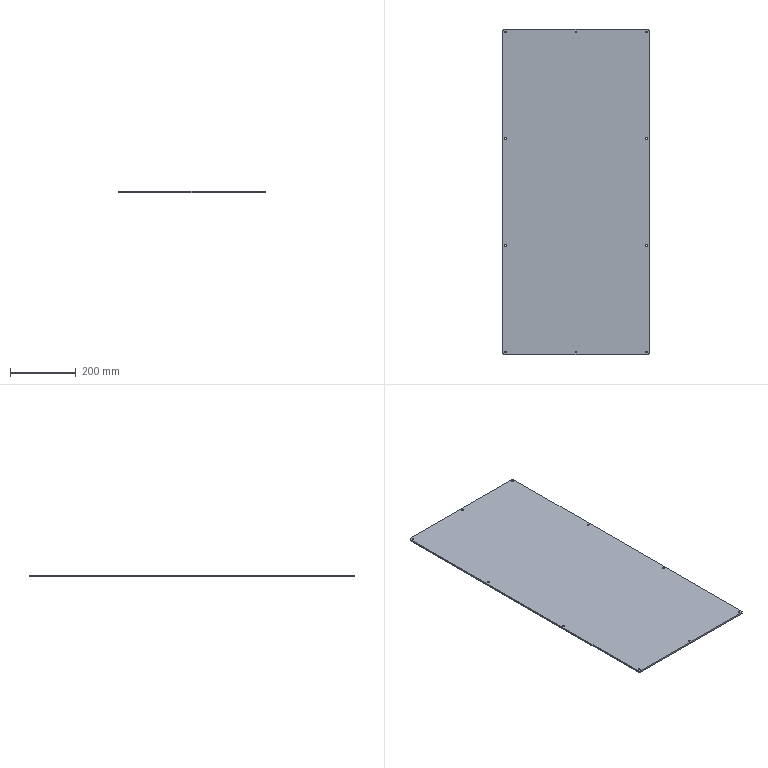Part | NX | features BREP 1 | 1 solid | 30 faces | box 446 x 992 x 5 mm | volume 2210732 mm3 | cylinder 24 | plane 6 | commonest cylinder face diameters 5.8 x20 10 x4
STEP:
#1=CARTESIAN_POINT('',(-218.,496.,5.));
#2=VERTEX_POINT('',#1);
#3=CARTESIAN_POINT('',(-223.,491.,5.));
#4=VERTEX_POINT('',#3);
#5=CARTESIAN_POINT('',(-218.,491.,5.));
#6=DIRECTION('',(0.,0.,1.));
#7=DIRECTION('',(1.,0.,0.));
#8=AXIS2_PLACEMENT_3D('',#5,#6,#7);
#9=CIRCLE('',#8,5.);
#10=EDGE_CURVE('',#2,#4,#9,.T.);
#11=ORIENTED_EDGE('',*,*,#10,.F.);
#12=CARTESIAN_POINT('',(-218.,496.,0.));
#13=VERTEX_POINT('',#12);
#14=CARTESIAN_POINT('',(-218.,496.,5.));
#15=DIRECTION('',(0.,0.,1.));
#16=VECTOR('',#15,1000.);
#17=LINE('',#14,#16);
#18=EDGE_CURVE('',#13,#2,#17,.T.);
#19=ORIENTED_EDGE('',*,*,#18,.F.);
#20=CARTESIAN_POINT('',(-223.,491.,0.));
#21=VERTEX_POINT('',#20);
#22=CARTESIAN_POINT('',(-218.,491.,0.));
#23=DIRECTION('',(0.,0.,-1.));
#24=DIRECTION('',(1.,0.,0.));
#25=AXIS2_PLACEMENT_3D('',#22,#23,#24);
#26=CIRCLE('',#25,5.);
#27=EDGE_CURVE('',#21,#13,#26,.T.);
#28=ORIENTED_EDGE('',*,*,#27,.F.);
#29=CARTESIAN_POINT('',(-223.,491.,5.));
#30=DIRECTION('',(0.,0.,-1.));
#31=VECTOR('',#30,1000.);
#32=LINE('',#29,#31);
#33=EDGE_CURVE('',#4,#21,#32,.T.);
#34=ORIENTED_EDGE('',*,*,#33,.F.);
#35=EDGE_LOOP('',(#11,#19,#28,#34));
#36=FACE_BOUND('',#35,.T.);
#37=CARTESIAN_POINT('',(-218.,491.,5.));
#38=DIRECTION('',(0.,0.,-1.));
#39=DIRECTION('',(-1.,0.,0.));
#40=AXIS2_PLACEMENT_3D('',#37,#38,#39);
#41=CYLINDRICAL_SURFACE('',#40,5.);
#42=ADVANCED_FACE('',(#36),#41,.T.);
#43=CARTESIAN_POINT('',(223.,491.,5.));
#44=VERTEX_POINT('',#43);
#45=CARTESIAN_POINT('',(218.,496.,5.));
#46=VERTEX_POINT('',#45);
#47=CARTESIAN_POINT('',(218.,491.,5.));
#48=DIRECTION('',(0.,0.,1.));
#49=DIRECTION('',(1.,0.,0.));
#50=AXIS2_PLACEMENT_3D('',#47,#48,#49);
#51=CIRCLE('',#50,5.);
#52=EDGE_CURVE('',#44,#46,#51,.T.);
#53=ORIENTED_EDGE('',*,*,#52,.F.);
#54=CARTESIAN_POINT('',(223.,491.,0.));
#55=VERTEX_POINT('',#54);
#56=CARTESIAN_POINT('',(223.,491.,5.));
#57=DIRECTION('',(0.,0.,1.));
#58=VECTOR('',#57,1000.);
#59=LINE('',#56,#58);
#60=EDGE_CURVE('',#55,#44,#59,.T.);
#61=ORIENTED_EDGE('',*,*,#60,.F.);
#62=CARTESIAN_POINT('',(218.,496.,0.));
#63=VERTEX_POINT('',#62);
#64=CARTESIAN_POINT('',(218.,491.,0.));
#65=DIRECTION('',(0.,0.,-1.));
#66=DIRECTION('',(1.,0.,0.));
#67=AXIS2_PLACEMENT_3D('',#64,#65,#66);
#68=CIRCLE('',#67,5.);
#69=EDGE_CURVE('',#63,#55,#68,.T.);
#70=ORIENTED_EDGE('',*,*,#69,.F.);
#71=CARTESIAN_POINT('',(218.,496.,5.));
#72=DIRECTION('',(0.,0.,-1.));
#73=VECTOR('',#72,1000.);
#74=LINE('',#71,#73);
#75=EDGE_CURVE('',#46,#63,#74,.T.);
#76=ORIENTED_EDGE('',*,*,#75,.F.);
#77=EDGE_LOOP('',(#53,#61,#70,#76));
#78=FACE_BOUND('',#77,.T.);
#79=CARTESIAN_POINT('',(218.,491.,5.));
#80=DIRECTION('',(0.,0.,-1.));
#81=DIRECTION('',(-1.,0.,0.));
#82=AXIS2_PLACEMENT_3D('',#79,#80,#81);
#83=CYLINDRICAL_SURFACE('',#82,5.);
#84=ADVANCED_FACE('',(#78),#83,.T.);
#85=CARTESIAN_POINT('',(218.,-496.,5.));
#86=VERTEX_POINT('',#85);
#87=CARTESIAN_POINT('',(223.,-491.,5.));
#88=VERTEX_POINT('',#87);
#89=CARTESIAN_POINT('',(218.,-491.,5.));
#90=DIRECTION('',(0.,0.,1.));
#91=DIRECTION('',(1.,0.,0.));
#92=AXIS2_PLACEMENT_3D('',#89,#90,#91);
#93=CIRCLE('',#92,5.);
#94=EDGE_CURVE('',#86,#88,#93,.T.);
#95=ORIENTED_EDGE('',*,*,#94,.F.);
#96=CARTESIAN_POINT('',(218.,-496.,0.));
#97=VERTEX_POINT('',#96);
#98=CARTESIAN_POINT('',(218.,-496.,5.));
#99=DIRECTION('',(0.,0.,1.));
#100=VECTOR('',#99,1000.);
#101=LINE('',#98,#100);
#102=EDGE_CURVE('',#97,#86,#101,.T.);
#103=ORIENTED_EDGE('',*,*,#102,.F.);
#104=CARTESIAN_POINT('',(223.,-491.,0.));
#105=VERTEX_POINT('',#104);
#106=CARTESIAN_POINT('',(218.,-491.,0.));
#107=DIRECTION('',(0.,0.,-1.));
#108=DIRECTION('',(1.,0.,0.));
#109=AXIS2_PLACEMENT_3D('',#106,#107,#108);
#110=CIRCLE('',#109,5.);
#111=EDGE_CURVE('',#105,#97,#110,.T.);
#112=ORIENTED_EDGE('',*,*,#111,.F.);
#113=CARTESIAN_POINT('',(223.,-491.,5.));
#114=DIRECTION('',(0.,0.,-1.));
#115=VECTOR('',#114,1000.);
#116=LINE('',#113,#115);
#117=EDGE_CURVE('',#88,#105,#116,.T.);
#118=ORIENTED_EDGE('',*,*,#117,.F.);
#119=EDGE_LOOP('',(#95,#103,#112,#118));
#120=FACE_BOUND('',#119,.T.);
#121=CARTESIAN_POINT('',(218.,-491.,5.));
#122=DIRECTION('',(0.,0.,-1.));
#123=DIRECTION('',(-1.,0.,0.));
#124=AXIS2_PLACEMENT_3D('',#121,#122,#123);
#125=CYLINDRICAL_SURFACE('',#124,5.);
#126=ADVANCED_FACE('',(#120),#125,.T.);
#127=CARTESIAN_POINT('',(-223.,-491.,5.));
#128=VERTEX_POINT('',#127);
#129=CARTESIAN_POINT('',(-218.,-496.,5.));
#130=VERTEX_POINT('',#129);
#131=CARTESIAN_POINT('',(-218.,-491.,5.));
#132=DIRECTION('',(0.,0.,1.));
#133=DIRECTION('',(1.,0.,0.));
#134=AXIS2_PLACEMENT_3D('',#131,#132,#133);
#135=CIRCLE('',#134,5.);
#136=EDGE_CURVE('',#128,#130,#135,.T.);
#137=ORIENTED_EDGE('',*,*,#136,.F.);
#138=CARTESIAN_POINT('',(-223.,-491.,0.));
#139=VERTEX_POINT('',#138);
#140=CARTESIAN_POINT('',(-223.,-491.,5.));
#141=DIRECTION('',(0.,0.,1.));
#142=VECTOR('',#141,1000.);
#143=LINE('',#140,#142);
#144=EDGE_CURVE('',#139,#128,#143,.T.);
#145=ORIENTED_EDGE('',*,*,#144,.F.);
#146=CARTESIAN_POINT('',(-218.,-496.,0.));
#147=VERTEX_POINT('',#146);
#148=CARTESIAN_POINT('',(-218.,-491.,0.));
#149=DIRECTION('',(0.,0.,-1.));
#150=DIRECTION('',(1.,0.,0.));
#151=AXIS2_PLACEMENT_3D('',#148,#149,#150);
#152=CIRCLE('',#151,5.);
#153=EDGE_CURVE('',#147,#139,#152,.T.);
#154=ORIENTED_EDGE('',*,*,#153,.F.);
#155=CARTESIAN_POINT('',(-218.,-496.,5.));
#156=DIRECTION('',(0.,0.,-1.));
#157=VECTOR('',#156,1000.);
#158=LINE('',#155,#157);
#159=EDGE_CURVE('',#130,#147,#158,.T.);
#160=ORIENTED_EDGE('',*,*,#159,.F.);
#161=EDGE_LOOP('',(#137,#145,#154,#160));
#162=FACE_BOUND('',#161,.T.);
#163=CARTESIAN_POINT('',(-218.,-491.,5.));
#164=DIRECTION('',(0.,0.,-1.));
#165=DIRECTION('',(-1.,0.,0.));
#166=AXIS2_PLACEMENT_3D('',#163,#164,#165);
#167=CYLINDRICAL_SURFACE('',#166,5.);
#168=ADVANCED_FACE('',(#162),#167,.T.);
#169=CARTESIAN_POINT('',(212.1,-488.,5.));
#170=VERTEX_POINT('',#169);
#171=CARTESIAN_POINT('',(212.1,-488.,0.));
#172=VERTEX_POINT('',#171);
#173=CARTESIAN_POINT('',(212.1,-488.,0.));
#174=DIRECTION('',(0.,0.,1.));
#175=VECTOR('',#174,1000.);
#176=LINE('',#173,#175);
#177=EDGE_CURVE('',#170,#172,#176,.F.);
#178=ORIENTED_EDGE('',*,*,#177,.T.);
#179=CARTESIAN_POINT('',(217.9,-488.,0.));
#180=VERTEX_POINT('',#179);
#181=CARTESIAN_POINT('',(215.,-488.,0.));
#182=DIRECTION('',(0.,0.,1.));
#183=DIRECTION('',(1.,0.,0.));
#184=AXIS2_PLACEMENT_3D('',#181,#182,#183);
#185=CIRCLE('',#184,2.9);
#186=EDGE_CURVE('',#180,#172,#185,.T.);
#187=ORIENTED_EDGE('',*,*,#186,.F.);
#188=CARTESIAN_POINT('',(217.9,-488.,5.));
#189=VERTEX_POINT('',#188);
#190=CARTESIAN_POINT('',(217.9,-488.,0.));
#191=DIRECTION('',(0.,0.,1.));
#192=VECTOR('',#191,1000.);
#193=LINE('',#190,#192);
#194=EDGE_CURVE('',#189,#180,#193,.F.);
#195=ORIENTED_EDGE('',*,*,#194,.F.);
#196=CARTESIAN_POINT('',(215.,-488.,5.));
#197=DIRECTION('',(0.,0.,1.));
#198=DIRECTION('',(1.,0.,0.));
#199=AXIS2_PLACEMENT_3D('',#196,#197,#198);
#200=CIRCLE('',#199,2.9);
#201=EDGE_CURVE('',#189,#170,#200,.T.);
#202=ORIENTED_EDGE('',*,*,#201,.T.);
#203=EDGE_LOOP('',(#178,#187,#195,#202));
#204=FACE_BOUND('',#203,.T.);
#205=CARTESIAN_POINT('',(215.,-488.,0.));
#206=DIRECTION('',(0.,0.,1.));
#207=DIRECTION('',(1.,0.,0.));
#208=AXIS2_PLACEMENT_3D('',#205,#206,#207);
#209=CYLINDRICAL_SURFACE('',#208,2.9);
#210=ADVANCED_FACE('',(#204),#209,.F.);
#211=CARTESIAN_POINT('',(212.1,162.667,5.));
#212=VERTEX_POINT('',#211);
#213=CARTESIAN_POINT('',(212.1,162.667,0.));
#214=VERTEX_POINT('',#213);
#215=CARTESIAN_POINT('',(212.1,162.667,0.));
#216=DIRECTION('',(0.,0.,1.));
#217=VECTOR('',#216,1000.);
#218=LINE('',#215,#217);
#219=EDGE_CURVE('',#212,#214,#218,.F.);
#220=ORIENTED_EDGE('',*,*,#219,.T.);
#221=CARTESIAN_POINT('',(217.9,162.667,0.));
#222=VERTEX_POINT('',#221);
#223=CARTESIAN_POINT('',(215.,162.667,0.));
#224=DIRECTION('',(0.,0.,1.));
#225=DIRECTION('',(1.,0.,0.));
#226=AXIS2_PLACEMENT_3D('',#223,#224,#225);
#227=CIRCLE('',#226,2.9);
#228=EDGE_CURVE('',#222,#214,#227,.T.);
#229=ORIENTED_EDGE('',*,*,#228,.F.);
#230=CARTESIAN_POINT('',(217.9,162.667,5.));
#231=VERTEX_POINT('',#230);
#232=CARTESIAN_POINT('',(217.9,162.667,0.));
#233=DIRECTION('',(0.,0.,1.));
#234=VECTOR('',#233,1000.);
#235=LINE('',#232,#234);
#236=EDGE_CURVE('',#231,#222,#235,.F.);
#237=ORIENTED_EDGE('',*,*,#236,.F.);
#238=CARTESIAN_POINT('',(215.,162.667,5.));
#239=DIRECTION('',(0.,0.,1.));
#240=DIRECTION('',(1.,0.,0.));
#241=AXIS2_PLACEMENT_3D('',#238,#239,#240);
#242=CIRCLE('',#241,2.9);
#243=EDGE_CURVE('',#231,#212,#242,.T.);
#244=ORIENTED_EDGE('',*,*,#243,.T.);
#245=EDGE_LOOP('',(#220,#229,#237,#244));
#246=FACE_BOUND('',#245,.T.);
#247=CARTESIAN_POINT('',(215.,162.667,0.));
#248=DIRECTION('',(0.,0.,1.));
#249=DIRECTION('',(1.,0.,0.));
#250=AXIS2_PLACEMENT_3D('',#247,#248,#249);
#251=CYLINDRICAL_SURFACE('',#250,2.9);
#252=ADVANCED_FACE('',(#246),#251,.F.);
#253=CARTESIAN_POINT('',(212.1,-162.667,5.));
#254=VERTEX_POINT('',#253);
#255=CARTESIAN_POINT('',(212.1,-162.667,0.));
#256=VERTEX_POINT('',#255);
#257=CARTESIAN_POINT('',(212.1,-162.667,0.));
#258=DIRECTION('',(0.,0.,1.));
#259=VECTOR('',#258,1000.);
#260=LINE('',#257,#259);
#261=EDGE_CURVE('',#254,#256,#260,.F.);
#262=ORIENTED_EDGE('',*,*,#261,.T.);
#263=CARTESIAN_POINT('',(217.9,-162.667,0.));
#264=VERTEX_POINT('',#263);
#265=CARTESIAN_POINT('',(215.,-162.667,0.));
#266=DIRECTION('',(0.,0.,1.));
#267=DIRECTION('',(1.,0.,0.));
#268=AXIS2_PLACEMENT_3D('',#265,#266,#267);
#269=CIRCLE('',#268,2.9);
#270=EDGE_CURVE('',#264,#256,#269,.T.);
#271=ORIENTED_EDGE('',*,*,#270,.F.);
#272=CARTESIAN_POINT('',(217.9,-162.667,5.));
#273=VERTEX_POINT('',#272);
#274=CARTESIAN_POINT('',(217.9,-162.667,0.));
#275=DIRECTION('',(0.,0.,1.));
#276=VECTOR('',#275,1000.);
#277=LINE('',#274,#276);
#278=EDGE_CURVE('',#273,#264,#277,.F.);
#279=ORIENTED_EDGE('',*,*,#278,.F.);
#280=CARTESIAN_POINT('',(215.,-162.667,5.));
#281=DIRECTION('',(0.,0.,1.));
#282=DIRECTION('',(1.,0.,0.));
#283=AXIS2_PLACEMENT_3D('',#280,#281,#282);
#284=CIRCLE('',#283,2.9);
#285=EDGE_CURVE('',#273,#254,#284,.T.);
#286=ORIENTED_EDGE('',*,*,#285,.T.);
#287=EDGE_LOOP('',(#262,#271,#279,#286));
#288=FACE_BOUND('',#287,.T.);
#289=CARTESIAN_POINT('',(215.,-162.667,0.));
#290=DIRECTION('',(0.,0.,1.));
#291=DIRECTION('',(1.,0.,0.));
#292=AXIS2_PLACEMENT_3D('',#289,#290,#291);
#293=CYLINDRICAL_SURFACE('',#292,2.9);
#294=ADVANCED_FACE('',(#288),#293,.F.);
#295=CARTESIAN_POINT('',(-217.9,162.667,5.));
#296=VERTEX_POINT('',#295);
#297=CARTESIAN_POINT('',(-217.9,162.667,0.));
#298=VERTEX_POINT('',#297);
#299=CARTESIAN_POINT('',(-217.9,162.667,0.));
#300=DIRECTION('',(0.,0.,1.));
#301=VECTOR('',#300,1000.);
#302=LINE('',#299,#301);
#303=EDGE_CURVE('',#296,#298,#302,.F.);
#304=ORIENTED_EDGE('',*,*,#303,.T.);
#305=CARTESIAN_POINT('',(-212.1,162.667,0.));
#306=VERTEX_POINT('',#305);
#307=CARTESIAN_POINT('',(-215.,162.667,0.));
#308=DIRECTION('',(0.,0.,1.));
#309=DIRECTION('',(1.,0.,0.));
#310=AXIS2_PLACEMENT_3D('',#307,#308,#309);
#311=CIRCLE('',#310,2.9);
#312=EDGE_CURVE('',#306,#298,#311,.T.);
#313=ORIENTED_EDGE('',*,*,#312,.F.);
#314=CARTESIAN_POINT('',(-212.1,162.667,5.));
#315=VERTEX_POINT('',#314);
#316=CARTESIAN_POINT('',(-212.1,162.667,0.));
#317=DIRECTION('',(0.,0.,1.));
#318=VECTOR('',#317,1000.);
#319=LINE('',#316,#318);
#320=EDGE_CURVE('',#315,#306,#319,.F.);
#321=ORIENTED_EDGE('',*,*,#320,.F.);
#322=CARTESIAN_POINT('',(-215.,162.667,5.));
#323=DIRECTION('',(0.,0.,1.));
#324=DIRECTION('',(1.,0.,0.));
#325=AXIS2_PLACEMENT_3D('',#322,#323,#324);
#326=CIRCLE('',#325,2.9);
#327=EDGE_CURVE('',#315,#296,#326,.T.);
#328=ORIENTED_EDGE('',*,*,#327,.T.);
#329=EDGE_LOOP('',(#304,#313,#321,#328));
#330=FACE_BOUND('',#329,.T.);
#331=CARTESIAN_POINT('',(-215.,162.667,0.));
#332=DIRECTION('',(0.,0.,1.));
#333=DIRECTION('',(1.,0.,0.));
#334=AXIS2_PLACEMENT_3D('',#331,#332,#333);
#335=CYLINDRICAL_SURFACE('',#334,2.9);
#336=ADVANCED_FACE('',(#330),#335,.F.);
#337=CARTESIAN_POINT('',(-2.9,-488.,5.));
#338=VERTEX_POINT('',#337);
#339=CARTESIAN_POINT('',(-2.9,-488.,0.));
#340=VERTEX_POINT('',#339);
#341=CARTESIAN_POINT('',(-2.9,-488.,0.));
#342=DIRECTION('',(0.,0.,1.));
#343=VECTOR('',#342,1000.);
#344=LINE('',#341,#343);
#345=EDGE_CURVE('',#338,#340,#344,.F.);
#346=ORIENTED_EDGE('',*,*,#345,.T.);
#347=CARTESIAN_POINT('',(2.9,-488.,0.));
#348=VERTEX_POINT('',#347);
#349=CARTESIAN_POINT('',(0.,-488.,0.));
#350=DIRECTION('',(0.,0.,1.));
#351=DIRECTION('',(1.,0.,0.));
#352=AXIS2_PLACEMENT_3D('',#349,#350,#351);
#353=CIRCLE('',#352,2.9);
#354=EDGE_CURVE('',#348,#340,#353,.T.);
#355=ORIENTED_EDGE('',*,*,#354,.F.);
#356=CARTESIAN_POINT('',(2.9,-488.,5.));
#357=VERTEX_POINT('',#356);
#358=CARTESIAN_POINT('',(2.9,-488.,0.));
#359=DIRECTION('',(0.,0.,1.));
#360=VECTOR('',#359,1000.);
#361=LINE('',#358,#360);
#362=EDGE_CURVE('',#357,#348,#361,.F.);
#363=ORIENTED_EDGE('',*,*,#362,.F.);
#364=CARTESIAN_POINT('',(0.,-488.,5.));
#365=DIRECTION('',(0.,0.,1.));
#366=DIRECTION('',(1.,0.,0.));
#367=AXIS2_PLACEMENT_3D('',#364,#365,#366);
#368=CIRCLE('',#367,2.9);
#369=EDGE_CURVE('',#357,#338,#368,.T.);
#370=ORIENTED_EDGE('',*,*,#369,.T.);
#371=EDGE_LOOP('',(#346,#355,#363,#370));
#372=FACE_BOUND('',#371,.T.);
#373=CARTESIAN_POINT('',(0.,-488.,0.));
#374=DIRECTION('',(0.,0.,1.));
#375=DIRECTION('',(1.,0.,0.));
#376=AXIS2_PLACEMENT_3D('',#373,#374,#375);
#377=CYLINDRICAL_SURFACE('',#376,2.9);
#378=ADVANCED_FACE('',(#372),#377,.F.);
#379=CARTESIAN_POINT('',(-217.9,-488.,5.));
#380=VERTEX_POINT('',#379);
#381=CARTESIAN_POINT('',(-217.9,-488.,0.));
#382=VERTEX_POINT('',#381);
#383=CARTESIAN_POINT('',(-217.9,-488.,0.));
#384=DIRECTION('',(0.,0.,1.));
#385=VECTOR('',#384,1000.);
#386=LINE('',#383,#385);
#387=EDGE_CURVE('',#380,#382,#386,.F.);
#388=ORIENTED_EDGE('',*,*,#387,.T.);
#389=CARTESIAN_POINT('',(-212.1,-488.,0.));
#390=VERTEX_POINT('',#389);
#391=CARTESIAN_POINT('',(-215.,-488.,0.));
#392=DIRECTION('',(0.,0.,1.));
#393=DIRECTION('',(1.,0.,0.));
#394=AXIS2_PLACEMENT_3D('',#391,#392,#393);
#395=CIRCLE('',#394,2.9);
#396=EDGE_CURVE('',#390,#382,#395,.T.);
#397=ORIENTED_EDGE('',*,*,#396,.F.);
#398=CARTESIAN_POINT('',(-212.1,-488.,5.));
#399=VERTEX_POINT('',#398);
#400=CARTESIAN_POINT('',(-212.1,-488.,0.));
#401=DIRECTION('',(0.,0.,1.));
#402=VECTOR('',#401,1000.);
#403=LINE('',#400,#402);
#404=EDGE_CURVE('',#399,#390,#403,.F.);
#405=ORIENTED_EDGE('',*,*,#404,.F.);
#406=CARTESIAN_POINT('',(-215.,-488.,5.));
#407=DIRECTION('',(0.,0.,1.));
#408=DIRECTION('',(1.,0.,0.));
#409=AXIS2_PLACEMENT_3D('',#406,#407,#408);
#410=CIRCLE('',#409,2.9);
#411=EDGE_CURVE('',#399,#380,#410,.T.);
#412=ORIENTED_EDGE('',*,*,#411,.T.);
#413=EDGE_LOOP('',(#388,#397,#405,#412));
#414=FACE_BOUND('',#413,.T.);
#415=CARTESIAN_POINT('',(-215.,-488.,0.));
#416=DIRECTION('',(0.,0.,1.));
#417=DIRECTION('',(1.,0.,0.));
#418=AXIS2_PLACEMENT_3D('',#415,#416,#417);
#419=CYLINDRICAL_SURFACE('',#418,2.9);
#420=ADVANCED_FACE('',(#414),#419,.F.);
#421=CARTESIAN_POINT('',(212.1,488.,5.));
#422=VERTEX_POINT('',#421);
#423=CARTESIAN_POINT('',(212.1,488.,0.));
#424=VERTEX_POINT('',#423);
#425=CARTESIAN_POINT('',(212.1,488.,0.));
#426=DIRECTION('',(0.,0.,1.));
#427=VECTOR('',#426,1000.);
#428=LINE('',#425,#427);
#429=EDGE_CURVE('',#422,#424,#428,.F.);
#430=ORIENTED_EDGE('',*,*,#429,.T.);
#431=CARTESIAN_POINT('',(217.9,488.,0.));
#432=VERTEX_POINT('',#431);
#433=CARTESIAN_POINT('',(215.,488.,0.));
#434=DIRECTION('',(0.,0.,1.));
#435=DIRECTION('',(1.,0.,0.));
#436=AXIS2_PLACEMENT_3D('',#433,#434,#435);
#437=CIRCLE('',#436,2.9);
#438=EDGE_CURVE('',#432,#424,#437,.T.);
#439=ORIENTED_EDGE('',*,*,#438,.F.);
#440=CARTESIAN_POINT('',(217.9,488.,5.));
#441=VERTEX_POINT('',#440);
#442=CARTESIAN_POINT('',(217.9,488.,0.));
#443=DIRECTION('',(0.,0.,1.));
#444=VECTOR('',#443,1000.);
#445=LINE('',#442,#444);
#446=EDGE_CURVE('',#441,#432,#445,.F.);
#447=ORIENTED_EDGE('',*,*,#446,.F.);
#448=CARTESIAN_POINT('',(215.,488.,5.));
#449=DIRECTION('',(0.,0.,1.));
#450=DIRECTION('',(1.,0.,0.));
#451=AXIS2_PLACEMENT_3D('',#448,#449,#450);
#452=CIRCLE('',#451,2.9);
#453=EDGE_CURVE('',#441,#422,#452,.T.);
#454=ORIENTED_EDGE('',*,*,#453,.T.);
#455=EDGE_LOOP('',(#430,#439,#447,#454));
#456=FACE_BOUND('',#455,.T.);
#457=CARTESIAN_POINT('',(215.,488.,0.));
#458=DIRECTION('',(0.,0.,1.));
#459=DIRECTION('',(1.,0.,0.));
#460=AXIS2_PLACEMENT_3D('',#457,#458,#459);
#461=CYLINDRICAL_SURFACE('',#460,2.9);
#462=ADVANCED_FACE('',(#456),#461,.F.);
#463=CARTESIAN_POINT('',(-2.9,488.,5.));
#464=VERTEX_POINT('',#463);
#465=CARTESIAN_POINT('',(-2.9,488.,0.));
#466=VERTEX_POINT('',#465);
#467=CARTESIAN_POINT('',(-2.9,488.,0.));
#468=DIRECTION('',(0.,0.,1.));
#469=VECTOR('',#468,1000.);
#470=LINE('',#467,#469);
#471=EDGE_CURVE('',#464,#466,#470,.F.);
#472=ORIENTED_EDGE('',*,*,#471,.T.);
#473=CARTESIAN_POINT('',(2.9,488.,0.));
#474=VERTEX_POINT('',#473);
#475=CARTESIAN_POINT('',(0.,488.,0.));
#476=DIRECTION('',(0.,0.,1.));
#477=DIRECTION('',(1.,0.,0.));
#478=AXIS2_PLACEMENT_3D('',#475,#476,#477);
#479=CIRCLE('',#478,2.9);
#480=EDGE_CURVE('',#474,#466,#479,.T.);
#481=ORIENTED_EDGE('',*,*,#480,.F.);
#482=CARTESIAN_POINT('',(2.9,488.,5.));
#483=VERTEX_POINT('',#482);
#484=CARTESIAN_POINT('',(2.9,488.,0.));
#485=DIRECTION('',(0.,0.,1.));
#486=VECTOR('',#485,1000.);
#487=LINE('',#484,#486);
#488=EDGE_CURVE('',#483,#474,#487,.F.);
#489=ORIENTED_EDGE('',*,*,#488,.F.);
#490=CARTESIAN_POINT('',(0.,488.,5.));
#491=DIRECTION('',(0.,0.,1.));
#492=DIRECTION('',(1.,0.,0.));
#493=AXIS2_PLACEMENT_3D('',#490,#491,#492);
#494=CIRCLE('',#493,2.9);
#495=EDGE_CURVE('',#483,#464,#494,.T.);
#496=ORIENTED_EDGE('',*,*,#495,.T.);
#497=EDGE_LOOP('',(#472,#481,#489,#496));
#498=FACE_BOUND('',#497,.T.);
#499=CARTESIAN_POINT('',(0.,488.,0.));
#500=DIRECTION('',(0.,0.,1.));
#501=DIRECTION('',(1.,0.,0.));
#502=AXIS2_PLACEMENT_3D('',#499,#500,#501);
#503=CYLINDRICAL_SURFACE('',#502,2.9);
#504=ADVANCED_FACE('',(#498),#503,.F.);
#505=CARTESIAN_POINT('',(-217.9,-162.667,5.));
#506=VERTEX_POINT('',#505);
#507=CARTESIAN_POINT('',(-217.9,-162.667,0.));
#508=VERTEX_POINT('',#507);
#509=CARTESIAN_POINT('',(-217.9,-162.667,0.));
#510=DIRECTION('',(0.,0.,1.));
#511=VECTOR('',#510,1000.);
#512=LINE('',#509,#511);
#513=EDGE_CURVE('',#506,#508,#512,.F.);
#514=ORIENTED_EDGE('',*,*,#513,.T.);
#515=CARTESIAN_POINT('',(-212.1,-162.667,0.));
#516=VERTEX_POINT('',#515);
#517=CARTESIAN_POINT('',(-215.,-162.667,0.));
#518=DIRECTION('',(0.,0.,1.));
#519=DIRECTION('',(1.,0.,0.));
#520=AXIS2_PLACEMENT_3D('',#517,#518,#519);
#521=CIRCLE('',#520,2.9);
#522=EDGE_CURVE('',#516,#508,#521,.T.);
#523=ORIENTED_EDGE('',*,*,#522,.F.);
#524=CARTESIAN_POINT('',(-212.1,-162.667,5.));
#525=VERTEX_POINT('',#524);
#526=CARTESIAN_POINT('',(-212.1,-162.667,0.));
#527=DIRECTION('',(0.,0.,1.));
#528=VECTOR('',#527,1000.);
#529=LINE('',#526,#528);
#530=EDGE_CURVE('',#525,#516,#529,.F.);
#531=ORIENTED_EDGE('',*,*,#530,.F.);
#532=CARTESIAN_POINT('',(-215.,-162.667,5.));
#533=DIRECTION('',(0.,0.,1.));
#534=DIRECTION('',(1.,0.,0.));
#535=AXIS2_PLACEMENT_3D('',#532,#533,#534);
#536=CIRCLE('',#535,2.9);
#537=EDGE_CURVE('',#525,#506,#536,.T.);
#538=ORIENTED_EDGE('',*,*,#537,.T.);
#539=EDGE_LOOP('',(#514,#523,#531,#538));
#540=FACE_BOUND('',#539,.T.);
#541=CARTESIAN_POINT('',(-215.,-162.667,0.));
#542=DIRECTION('',(0.,0.,1.));
#543=DIRECTION('',(1.,0.,0.));
#544=AXIS2_PLACEMENT_3D('',#541,#542,#543);
#545=CYLINDRICAL_SURFACE('',#544,2.9);
#546=ADVANCED_FACE('',(#540),#545,.F.);
#547=CARTESIAN_POINT('',(-217.9,488.,5.));
#548=VERTEX_POINT('',#547);
#549=CARTESIAN_POINT('',(-217.9,488.,0.));
#550=VERTEX_POINT('',#549);
#551=CARTESIAN_POINT('',(-217.9,488.,0.));
#552=DIRECTION('',(0.,0.,1.));
#553=VECTOR('',#552,1000.);
#554=LINE('',#551,#553);
#555=EDGE_CURVE('',#548,#550,#554,.F.);
#556=ORIENTED_EDGE('',*,*,#555,.T.);
#557=CARTESIAN_POINT('',(-212.1,488.,0.));
#558=VERTEX_POINT('',#557);
#559=CARTESIAN_POINT('',(-215.,488.,0.));
#560=DIRECTION('',(0.,0.,1.));
#561=DIRECTION('',(1.,0.,0.));
#562=AXIS2_PLACEMENT_3D('',#559,#560,#561);
#563=CIRCLE('',#562,2.9);
#564=EDGE_CURVE('',#558,#550,#563,.T.);
#565=ORIENTED_EDGE('',*,*,#564,.F.);
#566=CARTESIAN_POINT('',(-212.1,488.,5.));
#567=VERTEX_POINT('',#566);
#568=CARTESIAN_POINT('',(-212.1,488.,0.));
#569=DIRECTION('',(0.,0.,1.));
#570=VECTOR('',#569,1000.);
#571=LINE('',#568,#570);
#572=EDGE_CURVE('',#567,#558,#571,.F.);
#573=ORIENTED_EDGE('',*,*,#572,.F.);
#574=CARTESIAN_POINT('',(-215.,488.,5.));
#575=DIRECTION('',(0.,0.,1.));
#576=DIRECTION('',(1.,0.,0.));
#577=AXIS2_PLACEMENT_3D('',#574,#575,#576);
#578=CIRCLE('',#577,2.9);
#579=EDGE_CURVE('',#567,#548,#578,.T.);
#580=ORIENTED_EDGE('',*,*,#579,.T.);
#581=EDGE_LOOP('',(#556,#565,#573,#580));
#582=FACE_BOUND('',#581,.T.);
#583=CARTESIAN_POINT('',(-215.,488.,0.));
#584=DIRECTION('',(0.,0.,1.));
#585=DIRECTION('',(1.,0.,0.));
#586=AXIS2_PLACEMENT_3D('',#583,#584,#585);
#587=CYLINDRICAL_SURFACE('',#586,2.9);
#588=ADVANCED_FACE('',(#582),#587,.F.);
#589=CARTESIAN_POINT('',(223.,-496.,0.));
#590=DIRECTION('',(1.,0.,0.));
#591=VECTOR('',#590,1000.);
#592=LINE('',#589,#591);
#593=EDGE_CURVE('',#147,#97,#592,.T.);
#594=ORIENTED_EDGE('',*,*,#593,.F.);
#595=ORIENTED_EDGE('',*,*,#153,.T.);
#596=CARTESIAN_POINT('',(-223.,-496.,0.));
#597=DIRECTION('',(0.,-1.,0.));
#598=VECTOR('',#597,1000.);
#599=LINE('',#596,#598);
#600=EDGE_CURVE('',#21,#139,#599,.T.);
#601=ORIENTED_EDGE('',*,*,#600,.F.);
#602=ORIENTED_EDGE('',*,*,#27,.T.);
#603=CARTESIAN_POINT('',(223.,496.,0.));
#604=DIRECTION('',(-1.,0.,0.));
#605=VECTOR('',#604,1000.);
#606=LINE('',#603,#605);
#607=EDGE_CURVE('',#63,#13,#606,.T.);
#608=ORIENTED_EDGE('',*,*,#607,.F.);
#609=ORIENTED_EDGE('',*,*,#69,.T.);
#610=CARTESIAN_POINT('',(223.,-496.,0.));
#611=DIRECTION('',(0.,1.,0.));
#612=VECTOR('',#611,1000.);
#613=LINE('',#610,#612);
#614=EDGE_CURVE('',#105,#55,#613,.T.);
#615=ORIENTED_EDGE('',*,*,#614,.F.);
#616=ORIENTED_EDGE('',*,*,#111,.T.);
#617=EDGE_LOOP('',(#594,#595,#601,#602,#608,#609,#615,#616));
#618=FACE_BOUND('',#617,.T.);
#619=ORIENTED_EDGE('',*,*,#564,.T.);
#620=CARTESIAN_POINT('',(-215.,488.,0.));
#621=DIRECTION('',(0.,0.,1.));
#622=DIRECTION('',(1.,0.,0.));
#623=AXIS2_PLACEMENT_3D('',#620,#621,#622);
#624=CIRCLE('',#623,2.9);
#625=EDGE_CURVE('',#550,#558,#624,.T.);
#626=ORIENTED_EDGE('',*,*,#625,.T.);
#627=EDGE_LOOP('',(#619,#626));
#628=FACE_BOUND('',#627,.T.);
#629=ORIENTED_EDGE('',*,*,#522,.T.);
#630=CARTESIAN_POINT('',(-215.,-162.667,0.));
#631=DIRECTION('',(0.,0.,1.));
#632=DIRECTION('',(1.,0.,0.));
#633=AXIS2_PLACEMENT_3D('',#630,#631,#632);
#634=CIRCLE('',#633,2.9);
#635=EDGE_CURVE('',#508,#516,#634,.T.);
#636=ORIENTED_EDGE('',*,*,#635,.T.);
#637=EDGE_LOOP('',(#629,#636));
#638=FACE_BOUND('',#637,.T.);
#639=ORIENTED_EDGE('',*,*,#480,.T.);
#640=CARTESIAN_POINT('',(0.,488.,0.));
#641=DIRECTION('',(0.,0.,1.));
#642=DIRECTION('',(1.,0.,0.));
#643=AXIS2_PLACEMENT_3D('',#640,#641,#642);
#644=CIRCLE('',#643,2.9);
#645=EDGE_CURVE('',#466,#474,#644,.T.);
#646=ORIENTED_EDGE('',*,*,#645,.T.);
#647=EDGE_LOOP('',(#639,#646));
#648=FACE_BOUND('',#647,.T.);
#649=ORIENTED_EDGE('',*,*,#438,.T.);
#650=CARTESIAN_POINT('',(215.,488.,0.));
#651=DIRECTION('',(0.,0.,1.));
#652=DIRECTION('',(1.,0.,0.));
#653=AXIS2_PLACEMENT_3D('',#650,#651,#652);
#654=CIRCLE('',#653,2.9);
#655=EDGE_CURVE('',#424,#432,#654,.T.);
#656=ORIENTED_EDGE('',*,*,#655,.T.);
#657=EDGE_LOOP('',(#649,#656));
#658=FACE_BOUND('',#657,.T.);
#659=ORIENTED_EDGE('',*,*,#396,.T.);
#660=CARTESIAN_POINT('',(-215.,-488.,0.));
#661=DIRECTION('',(0.,0.,1.));
#662=DIRECTION('',(1.,0.,0.));
#663=AXIS2_PLACEMENT_3D('',#660,#661,#662);
#664=CIRCLE('',#663,2.9);
#665=EDGE_CURVE('',#382,#390,#664,.T.);
#666=ORIENTED_EDGE('',*,*,#665,.T.);
#667=EDGE_LOOP('',(#659,#666));
#668=FACE_BOUND('',#667,.T.);
#669=ORIENTED_EDGE('',*,*,#354,.T.);
#670=CARTESIAN_POINT('',(0.,-488.,0.));
#671=DIRECTION('',(0.,0.,1.));
#672=DIRECTION('',(1.,0.,0.));
#673=AXIS2_PLACEMENT_3D('',#670,#671,#672);
#674=CIRCLE('',#673,2.9);
#675=EDGE_CURVE('',#340,#348,#674,.T.);
#676=ORIENTED_EDGE('',*,*,#675,.T.);
#677=EDGE_LOOP('',(#669,#676));
#678=FACE_BOUND('',#677,.T.);
#679=ORIENTED_EDGE('',*,*,#312,.T.);
#680=CARTESIAN_POINT('',(-215.,162.667,0.));
#681=DIRECTION('',(0.,0.,1.));
#682=DIRECTION('',(1.,0.,0.));
#683=AXIS2_PLACEMENT_3D('',#680,#681,#682);
#684=CIRCLE('',#683,2.9);
#685=EDGE_CURVE('',#298,#306,#684,.T.);
#686=ORIENTED_EDGE('',*,*,#685,.T.);
#687=EDGE_LOOP('',(#679,#686));
#688=FACE_BOUND('',#687,.T.);
#689=ORIENTED_EDGE('',*,*,#270,.T.);
#690=CARTESIAN_POINT('',(215.,-162.667,0.));
#691=DIRECTION('',(0.,0.,1.));
#692=DIRECTION('',(1.,0.,0.));
#693=AXIS2_PLACEMENT_3D('',#690,#691,#692);
#694=CIRCLE('',#693,2.9);
#695=EDGE_CURVE('',#256,#264,#694,.T.);
#696=ORIENTED_EDGE('',*,*,#695,.T.);
#697=EDGE_LOOP('',(#689,#696));
#698=FACE_BOUND('',#697,.T.);
#699=ORIENTED_EDGE('',*,*,#228,.T.);
#700=CARTESIAN_POINT('',(215.,162.667,0.));
#701=DIRECTION('',(0.,0.,1.));
#702=DIRECTION('',(1.,0.,0.));
#703=AXIS2_PLACEMENT_3D('',#700,#701,#702);
#704=CIRCLE('',#703,2.9);
#705=EDGE_CURVE('',#214,#222,#704,.T.);
#706=ORIENTED_EDGE('',*,*,#705,.T.);
#707=EDGE_LOOP('',(#699,#706));
#708=FACE_BOUND('',#707,.T.);
#709=ORIENTED_EDGE('',*,*,#186,.T.);
#710=CARTESIAN_POINT('',(215.,-488.,0.));
#711=DIRECTION('',(0.,0.,1.));
#712=DIRECTION('',(1.,0.,0.));
#713=AXIS2_PLACEMENT_3D('',#710,#711,#712);
#714=CIRCLE('',#713,2.9);
#715=EDGE_CURVE('',#172,#180,#714,.T.);
#716=ORIENTED_EDGE('',*,*,#715,.T.);
#717=EDGE_LOOP('',(#709,#716));
#718=FACE_BOUND('',#717,.T.);
#719=CARTESIAN_POINT('',(0.,0.,0.));
#720=DIRECTION('',(0.,0.,1.));
#721=DIRECTION('',(1.,0.,0.));
#722=AXIS2_PLACEMENT_3D('',#719,#720,#721);
#723=PLANE('',#722);
#724=ADVANCED_FACE('',(#618,#628,#638,#648,#658,#668,#678,#688,#698,#708,#718),#723,.F.);
#725=CARTESIAN_POINT('',(-223.,-496.,5.));
#726=DIRECTION('',(0.,-1.,0.));
#727=VECTOR('',#726,1000.);
#728=LINE('',#725,#727);
#729=EDGE_CURVE('',#4,#128,#728,.T.);
#730=ORIENTED_EDGE('',*,*,#729,.T.);
#731=ORIENTED_EDGE('',*,*,#136,.T.);
#732=CARTESIAN_POINT('',(223.,-496.,5.));
#733=DIRECTION('',(1.,0.,0.));
#734=VECTOR('',#733,1000.);
#735=LINE('',#732,#734);
#736=EDGE_CURVE('',#130,#86,#735,.T.);
#737=ORIENTED_EDGE('',*,*,#736,.T.);
#738=ORIENTED_EDGE('',*,*,#94,.T.);
#739=CARTESIAN_POINT('',(223.,-496.,5.));
#740=DIRECTION('',(0.,1.,0.));
#741=VECTOR('',#740,1000.);
#742=LINE('',#739,#741);
#743=EDGE_CURVE('',#88,#44,#742,.T.);
#744=ORIENTED_EDGE('',*,*,#743,.T.);
#745=ORIENTED_EDGE('',*,*,#52,.T.);
#746=CARTESIAN_POINT('',(223.,496.,5.));
#747=DIRECTION('',(-1.,0.,0.));
#748=VECTOR('',#747,1000.);
#749=LINE('',#746,#748);
#750=EDGE_CURVE('',#46,#2,#749,.T.);
#751=ORIENTED_EDGE('',*,*,#750,.T.);
#752=ORIENTED_EDGE('',*,*,#10,.T.);
#753=EDGE_LOOP('',(#730,#731,#737,#738,#744,#745,#751,#752));
#754=FACE_BOUND('',#753,.T.);
#755=ORIENTED_EDGE('',*,*,#579,.F.);
#756=CARTESIAN_POINT('',(-215.,488.,5.));
#757=DIRECTION('',(0.,0.,1.));
#758=DIRECTION('',(1.,0.,0.));
#759=AXIS2_PLACEMENT_3D('',#756,#757,#758);
#760=CIRCLE('',#759,2.9);
#761=EDGE_CURVE('',#548,#567,#760,.T.);
#762=ORIENTED_EDGE('',*,*,#761,.F.);
#763=EDGE_LOOP('',(#755,#762));
#764=FACE_BOUND('',#763,.T.);
#765=ORIENTED_EDGE('',*,*,#537,.F.);
#766=CARTESIAN_POINT('',(-215.,-162.667,5.));
#767=DIRECTION('',(0.,0.,1.));
#768=DIRECTION('',(1.,0.,0.));
#769=AXIS2_PLACEMENT_3D('',#766,#767,#768);
#770=CIRCLE('',#769,2.9);
#771=EDGE_CURVE('',#506,#525,#770,.T.);
#772=ORIENTED_EDGE('',*,*,#771,.F.);
#773=EDGE_LOOP('',(#765,#772));
#774=FACE_BOUND('',#773,.T.);
#775=ORIENTED_EDGE('',*,*,#495,.F.);
#776=CARTESIAN_POINT('',(0.,488.,5.));
#777=DIRECTION('',(0.,0.,1.));
#778=DIRECTION('',(1.,0.,0.));
#779=AXIS2_PLACEMENT_3D('',#776,#777,#778);
#780=CIRCLE('',#779,2.9);
#781=EDGE_CURVE('',#464,#483,#780,.T.);
#782=ORIENTED_EDGE('',*,*,#781,.F.);
#783=EDGE_LOOP('',(#775,#782));
#784=FACE_BOUND('',#783,.T.);
#785=ORIENTED_EDGE('',*,*,#453,.F.);
#786=CARTESIAN_POINT('',(215.,488.,5.));
#787=DIRECTION('',(0.,0.,1.));
#788=DIRECTION('',(1.,0.,0.));
#789=AXIS2_PLACEMENT_3D('',#786,#787,#788);
#790=CIRCLE('',#789,2.9);
#791=EDGE_CURVE('',#422,#441,#790,.T.);
#792=ORIENTED_EDGE('',*,*,#791,.F.);
#793=EDGE_LOOP('',(#785,#792));
#794=FACE_BOUND('',#793,.T.);
#795=ORIENTED_EDGE('',*,*,#411,.F.);
#796=CARTESIAN_POINT('',(-215.,-488.,5.));
#797=DIRECTION('',(0.,0.,1.));
#798=DIRECTION('',(1.,0.,0.));
#799=AXIS2_PLACEMENT_3D('',#796,#797,#798);
#800=CIRCLE('',#799,2.9);
#801=EDGE_CURVE('',#380,#399,#800,.T.);
#802=ORIENTED_EDGE('',*,*,#801,.F.);
#803=EDGE_LOOP('',(#795,#802));
#804=FACE_BOUND('',#803,.T.);
#805=ORIENTED_EDGE('',*,*,#369,.F.);
#806=CARTESIAN_POINT('',(0.,-488.,5.));
#807=DIRECTION('',(0.,0.,1.));
#808=DIRECTION('',(1.,0.,0.));
#809=AXIS2_PLACEMENT_3D('',#806,#807,#808);
#810=CIRCLE('',#809,2.9);
#811=EDGE_CURVE('',#338,#357,#810,.T.);
#812=ORIENTED_EDGE('',*,*,#811,.F.);
#813=EDGE_LOOP('',(#805,#812));
#814=FACE_BOUND('',#813,.T.);
#815=ORIENTED_EDGE('',*,*,#327,.F.);
#816=CARTESIAN_POINT('',(-215.,162.667,5.));
#817=DIRECTION('',(0.,0.,1.));
#818=DIRECTION('',(1.,0.,0.));
#819=AXIS2_PLACEMENT_3D('',#816,#817,#818);
#820=CIRCLE('',#819,2.9);
#821=EDGE_CURVE('',#296,#315,#820,.T.);
#822=ORIENTED_EDGE('',*,*,#821,.F.);
#823=EDGE_LOOP('',(#815,#822));
#824=FACE_BOUND('',#823,.T.);
#825=ORIENTED_EDGE('',*,*,#285,.F.);
#826=CARTESIAN_POINT('',(215.,-162.667,5.));
#827=DIRECTION('',(0.,0.,1.));
#828=DIRECTION('',(1.,0.,0.));
#829=AXIS2_PLACEMENT_3D('',#826,#827,#828);
#830=CIRCLE('',#829,2.9);
#831=EDGE_CURVE('',#254,#273,#830,.T.);
#832=ORIENTED_EDGE('',*,*,#831,.F.);
#833=EDGE_LOOP('',(#825,#832));
#834=FACE_BOUND('',#833,.T.);
#835=ORIENTED_EDGE('',*,*,#243,.F.);
#836=CARTESIAN_POINT('',(215.,162.667,5.));
#837=DIRECTION('',(0.,0.,1.));
#838=DIRECTION('',(1.,0.,0.));
#839=AXIS2_PLACEMENT_3D('',#836,#837,#838);
#840=CIRCLE('',#839,2.9);
#841=EDGE_CURVE('',#212,#231,#840,.T.);
#842=ORIENTED_EDGE('',*,*,#841,.F.);
#843=EDGE_LOOP('',(#835,#842));
#844=FACE_BOUND('',#843,.T.);
#845=ORIENTED_EDGE('',*,*,#201,.F.);
#846=CARTESIAN_POINT('',(215.,-488.,5.));
#847=DIRECTION('',(0.,0.,1.));
#848=DIRECTION('',(1.,0.,0.));
#849=AXIS2_PLACEMENT_3D('',#846,#847,#848);
#850=CIRCLE('',#849,2.9);
#851=EDGE_CURVE('',#170,#189,#850,.T.);
#852=ORIENTED_EDGE('',*,*,#851,.F.);
#853=EDGE_LOOP('',(#845,#852));
#854=FACE_BOUND('',#853,.T.);
#855=CARTESIAN_POINT('',(0.,0.,5.));
#856=DIRECTION('',(0.,0.,1.));
#857=DIRECTION('',(1.,0.,0.));
#858=AXIS2_PLACEMENT_3D('',#855,#856,#857);
#859=PLANE('',#858);
#860=ADVANCED_FACE('',(#754,#764,#774,#784,#794,#804,#814,#824,#834,#844,#854),#859,.T.);
#861=ORIENTED_EDGE('',*,*,#750,.F.);
#862=ORIENTED_EDGE('',*,*,#75,.T.);
#863=ORIENTED_EDGE('',*,*,#607,.T.);
#864=ORIENTED_EDGE('',*,*,#18,.T.);
#865=EDGE_LOOP('',(#861,#862,#863,#864));
#866=FACE_BOUND('',#865,.T.);
#867=CARTESIAN_POINT('',(223.,496.,5.));
#868=DIRECTION('',(0.,-1.,0.));
#869=DIRECTION('',(0.,0.,-1.));
#870=AXIS2_PLACEMENT_3D('',#867,#868,#869);
#871=PLANE('',#870);
#872=ADVANCED_FACE('',(#866),#871,.F.);
#873=ORIENTED_EDGE('',*,*,#743,.F.);
#874=ORIENTED_EDGE('',*,*,#117,.T.);
#875=ORIENTED_EDGE('',*,*,#614,.T.);
#876=ORIENTED_EDGE('',*,*,#60,.T.);
#877=EDGE_LOOP('',(#873,#874,#875,#876));
#878=FACE_BOUND('',#877,.T.);
#879=CARTESIAN_POINT('',(223.,-496.,5.));
#880=DIRECTION('',(-1.,0.,0.));
#881=DIRECTION('',(0.,0.,1.));
#882=AXIS2_PLACEMENT_3D('',#879,#880,#881);
#883=PLANE('',#882);
#884=ADVANCED_FACE('',(#878),#883,.F.);
#885=ORIENTED_EDGE('',*,*,#736,.F.);
#886=ORIENTED_EDGE('',*,*,#159,.T.);
#887=ORIENTED_EDGE('',*,*,#593,.T.);
#888=ORIENTED_EDGE('',*,*,#102,.T.);
#889=EDGE_LOOP('',(#885,#886,#887,#888));
#890=FACE_BOUND('',#889,.T.);
#891=CARTESIAN_POINT('',(223.,-496.,5.));
#892=DIRECTION('',(0.,1.,0.));
#893=DIRECTION('',(0.,0.,1.));
#894=AXIS2_PLACEMENT_3D('',#891,#892,#893);
#895=PLANE('',#894);
#896=ADVANCED_FACE('',(#890),#895,.F.);
#897=ORIENTED_EDGE('',*,*,#600,.T.);
#898=ORIENTED_EDGE('',*,*,#144,.T.);
#899=ORIENTED_EDGE('',*,*,#729,.F.);
#900=ORIENTED_EDGE('',*,*,#33,.T.);
#901=EDGE_LOOP('',(#897,#898,#899,#900));
#902=FACE_BOUND('',#901,.T.);
#903=CARTESIAN_POINT('',(-223.,-496.,5.));
#904=DIRECTION('',(1.,0.,0.));
#905=DIRECTION('',(0.,0.,-1.));
#906=AXIS2_PLACEMENT_3D('',#903,#904,#905);
#907=PLANE('',#906);
#908=ADVANCED_FACE('',(#902),#907,.F.);
#909=ORIENTED_EDGE('',*,*,#625,.F.);
#910=ORIENTED_EDGE('',*,*,#555,.F.);
#911=ORIENTED_EDGE('',*,*,#761,.T.);
#912=ORIENTED_EDGE('',*,*,#572,.T.);
#913=EDGE_LOOP('',(#909,#910,#911,#912));
#914=FACE_BOUND('',#913,.T.);
#915=CARTESIAN_POINT('',(-215.,488.,0.));
#916=DIRECTION('',(0.,0.,1.));
#917=DIRECTION('',(1.,0.,0.));
#918=AXIS2_PLACEMENT_3D('',#915,#916,#917);
#919=CYLINDRICAL_SURFACE('',#918,2.9);
#920=ADVANCED_FACE('',(#914),#919,.F.);
#921=ORIENTED_EDGE('',*,*,#635,.F.);
#922=ORIENTED_EDGE('',*,*,#513,.F.);
#923=ORIENTED_EDGE('',*,*,#771,.T.);
#924=ORIENTED_EDGE('',*,*,#530,.T.);
#925=EDGE_LOOP('',(#921,#922,#923,#924));
#926=FACE_BOUND('',#925,.T.);
#927=CARTESIAN_POINT('',(-215.,-162.667,0.));
#928=DIRECTION('',(0.,0.,1.));
#929=DIRECTION('',(1.,0.,0.));
#930=AXIS2_PLACEMENT_3D('',#927,#928,#929);
#931=CYLINDRICAL_SURFACE('',#930,2.9);
#932=ADVANCED_FACE('',(#926),#931,.F.);
#933=ORIENTED_EDGE('',*,*,#645,.F.);
#934=ORIENTED_EDGE('',*,*,#471,.F.);
#935=ORIENTED_EDGE('',*,*,#781,.T.);
#936=ORIENTED_EDGE('',*,*,#488,.T.);
#937=EDGE_LOOP('',(#933,#934,#935,#936));
#938=FACE_BOUND('',#937,.T.);
#939=CARTESIAN_POINT('',(0.,488.,0.));
#940=DIRECTION('',(0.,0.,1.));
#941=DIRECTION('',(1.,0.,0.));
#942=AXIS2_PLACEMENT_3D('',#939,#940,#941);
#943=CYLINDRICAL_SURFACE('',#942,2.9);
#944=ADVANCED_FACE('',(#938),#943,.F.);
#945=ORIENTED_EDGE('',*,*,#655,.F.);
#946=ORIENTED_EDGE('',*,*,#429,.F.);
#947=ORIENTED_EDGE('',*,*,#791,.T.);
#948=ORIENTED_EDGE('',*,*,#446,.T.);
#949=EDGE_LOOP('',(#945,#946,#947,#948));
#950=FACE_BOUND('',#949,.T.);
#951=CARTESIAN_POINT('',(215.,488.,0.));
#952=DIRECTION('',(0.,0.,1.));
#953=DIRECTION('',(1.,0.,0.));
#954=AXIS2_PLACEMENT_3D('',#951,#952,#953);
#955=CYLINDRICAL_SURFACE('',#954,2.9);
#956=ADVANCED_FACE('',(#950),#955,.F.);
#957=ORIENTED_EDGE('',*,*,#665,.F.);
#958=ORIENTED_EDGE('',*,*,#387,.F.);
#959=ORIENTED_EDGE('',*,*,#801,.T.);
#960=ORIENTED_EDGE('',*,*,#404,.T.);
#961=EDGE_LOOP('',(#957,#958,#959,#960));
#962=FACE_BOUND('',#961,.T.);
#963=CARTESIAN_POINT('',(-215.,-488.,0.));
#964=DIRECTION('',(0.,0.,1.));
#965=DIRECTION('',(1.,0.,0.));
#966=AXIS2_PLACEMENT_3D('',#963,#964,#965);
#967=CYLINDRICAL_SURFACE('',#966,2.9);
#968=ADVANCED_FACE('',(#962),#967,.F.);
#969=ORIENTED_EDGE('',*,*,#675,.F.);
#970=ORIENTED_EDGE('',*,*,#345,.F.);
#971=ORIENTED_EDGE('',*,*,#811,.T.);
#972=ORIENTED_EDGE('',*,*,#362,.T.);
#973=EDGE_LOOP('',(#969,#970,#971,#972));
#974=FACE_BOUND('',#973,.T.);
#975=CARTESIAN_POINT('',(0.,-488.,0.));
#976=DIRECTION('',(0.,0.,1.));
#977=DIRECTION('',(1.,0.,0.));
#978=AXIS2_PLACEMENT_3D('',#975,#976,#977);
#979=CYLINDRICAL_SURFACE('',#978,2.9);
#980=ADVANCED_FACE('',(#974),#979,.F.);
#981=ORIENTED_EDGE('',*,*,#685,.F.);
#982=ORIENTED_EDGE('',*,*,#303,.F.);
#983=ORIENTED_EDGE('',*,*,#821,.T.);
#984=ORIENTED_EDGE('',*,*,#320,.T.);
#985=EDGE_LOOP('',(#981,#982,#983,#984));
#986=FACE_BOUND('',#985,.T.);
#987=CARTESIAN_POINT('',(-215.,162.667,0.));
#988=DIRECTION('',(0.,0.,1.));
#989=DIRECTION('',(1.,0.,0.));
#990=AXIS2_PLACEMENT_3D('',#987,#988,#989);
#991=CYLINDRICAL_SURFACE('',#990,2.9);
#992=ADVANCED_FACE('',(#986),#991,.F.);
#993=ORIENTED_EDGE('',*,*,#695,.F.);
#994=ORIENTED_EDGE('',*,*,#261,.F.);
#995=ORIENTED_EDGE('',*,*,#831,.T.);
#996=ORIENTED_EDGE('',*,*,#278,.T.);
#997=EDGE_LOOP('',(#993,#994,#995,#996));
#998=FACE_BOUND('',#997,.T.);
#999=CARTESIAN_POINT('',(215.,-162.667,0.));
#1000=DIRECTION('',(0.,0.,1.));
#1001=DIRECTION('',(1.,0.,0.));
#1002=AXIS2_PLACEMENT_3D('',#999,#1000,#1001);
#1003=CYLINDRICAL_SURFACE('',#1002,2.9);
#1004=ADVANCED_FACE('',(#998),#1003,.F.);
#1005=ORIENTED_EDGE('',*,*,#705,.F.);
#1006=ORIENTED_EDGE('',*,*,#219,.F.);
#1007=ORIENTED_EDGE('',*,*,#841,.T.);
#1008=ORIENTED_EDGE('',*,*,#236,.T.);
#1009=EDGE_LOOP('',(#1005,#1006,#1007,#1008));
#1010=FACE_BOUND('',#1009,.T.);
#1011=CARTESIAN_POINT('',(215.,162.667,0.));
#1012=DIRECTION('',(0.,0.,1.));
#1013=DIRECTION('',(1.,0.,0.));
#1014=AXIS2_PLACEMENT_3D('',#1011,#1012,#1013);
#1015=CYLINDRICAL_SURFACE('',#1014,2.9);
#1016=ADVANCED_FACE('',(#1010),#1015,.F.);
#1017=ORIENTED_EDGE('',*,*,#715,.F.);
#1018=ORIENTED_EDGE('',*,*,#177,.F.);
#1019=ORIENTED_EDGE('',*,*,#851,.T.);
#1020=ORIENTED_EDGE('',*,*,#194,.T.);
#1021=EDGE_LOOP('',(#1017,#1018,#1019,#1020));
#1022=FACE_BOUND('',#1021,.T.);
#1023=CARTESIAN_POINT('',(215.,-488.,0.));
#1024=DIRECTION('',(0.,0.,1.));
#1025=DIRECTION('',(1.,0.,0.));
#1026=AXIS2_PLACEMENT_3D('',#1023,#1024,#1025);
#1027=CYLINDRICAL_SURFACE('',#1026,2.9);
#1028=ADVANCED_FACE('',(#1022),#1027,.F.);
#1029=CLOSED_SHELL('',(#42,#84,#126,#168,#210,#252,#294,#336,#378,#420,#462,#504,#546,#588,#724,#860,#872,#884,#896,#908,#920,#932,#944,#956,#968,#980,#992,#1004,#1016,#1028));
#1030=MANIFOLD_SOLID_BREP('',#1029);
#1031=(LENGTH_UNIT()NAMED_UNIT(*)SI_UNIT(.MILLI.,.METRE.));
#1032=UNCERTAINTY_MEASURE_WITH_UNIT(LENGTH_MEASURE(0.00001),#1031,'','');
#1033=(NAMED_UNIT(*)PLANE_ANGLE_UNIT()SI_UNIT($,.RADIAN.));
#1034=(NAMED_UNIT(*)SI_UNIT($,.STERADIAN.)SOLID_ANGLE_UNIT());
#1035=(GEOMETRIC_REPRESENTATION_CONTEXT(3)GLOBAL_UNCERTAINTY_ASSIGNED_CONTEXT((#1032))GLOBAL_UNIT_ASSIGNED_CONTEXT((#1031,#1033,#1034))REPRESENTATION_CONTEXT('',''));
#1036=ADVANCED_BREP_SHAPE_REPRESENTATION('',(#1030),#1035);